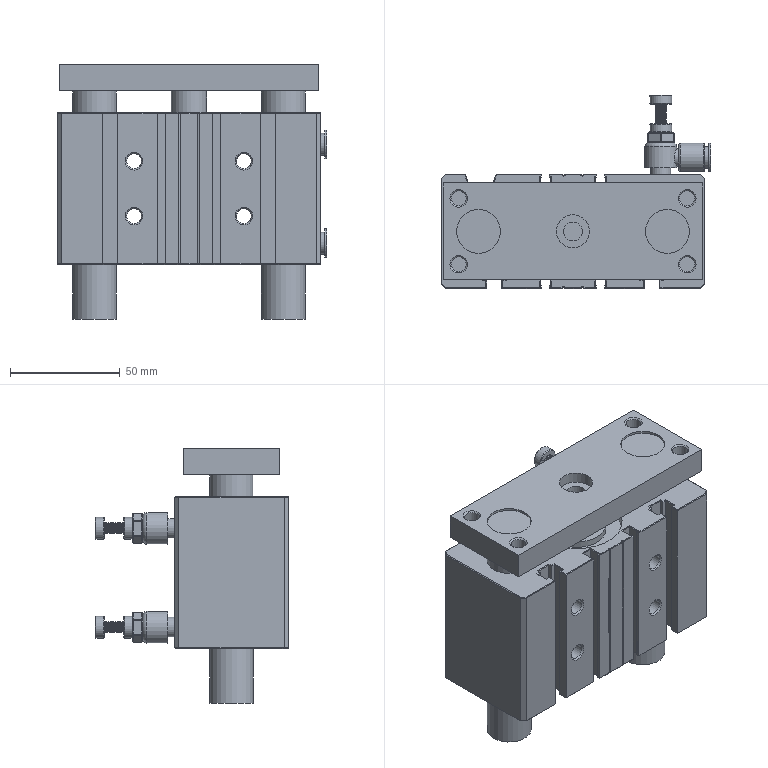Part | STEP file | Tube feed_id898_x_t | 1 solid | 429 faces | box 122.75 x 88 x 116 mm | volume 476709 mm3 | plane 336 | cylinder 53 | cone 28 | spline 6 | torus 6 | commonest cylinder face diameters 6.8 x12 10 x6 20 x6 1 x4 11 x4 13 x4